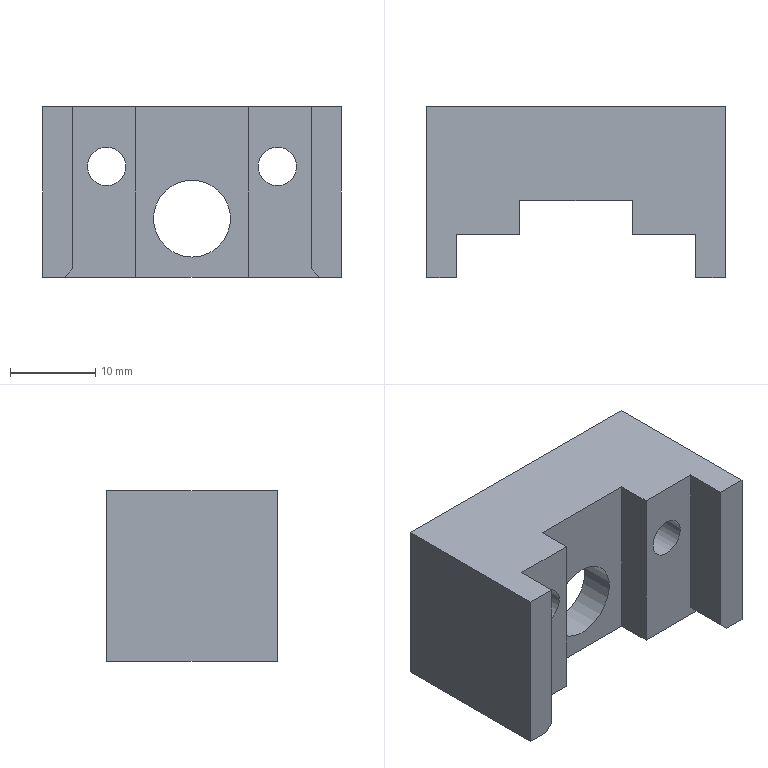Part | NX | features BREP 1 | 1 solid | 27 faces | box 35 x 20 x 20 mm | volume 7593 mm3 | plane 22 | cylinder 5 | commonest cylinder face diameters 4.5 x2 8 x2 9 x1
STEP:
#1=CARTESIAN_POINT('',(10.,-5.,-0.75));
#2=VERTEX_POINT('',#1);
#3=CARTESIAN_POINT('',(10.,-5.,-3.));
#4=DIRECTION('',(0.,1.,0.));
#5=DIRECTION('',(0.,0.,1.));
#6=AXIS2_PLACEMENT_3D('',#3,#4,#5);
#7=CIRCLE('',#6,2.25);
#8=EDGE_CURVE('',#2,#2,#7,.T.);
#9=ORIENTED_EDGE('',*,*,#8,.T.);
#10=EDGE_LOOP('',(#9));
#11=FACE_BOUND('',#10,.T.);
#12=CARTESIAN_POINT('',(14.,-5.,4.));
#13=VERTEX_POINT('',#12);
#14=CARTESIAN_POINT('',(6.6,-5.,4.));
#15=VERTEX_POINT('',#14);
#16=CARTESIAN_POINT('',(14.,-5.,4.));
#17=DIRECTION('',(-1.,0.,0.));
#18=VECTOR('',#17,1000.);
#19=LINE('',#16,#18);
#20=EDGE_CURVE('',#13,#15,#19,.T.);
#21=ORIENTED_EDGE('',*,*,#20,.T.);
#22=CARTESIAN_POINT('',(6.6,-5.,-16.));
#23=VERTEX_POINT('',#22);
#24=CARTESIAN_POINT('',(6.6,-5.,-16.));
#25=DIRECTION('',(0.,0.,1.));
#26=VECTOR('',#25,1000.);
#27=LINE('',#24,#26);
#28=EDGE_CURVE('',#23,#15,#27,.T.);
#29=ORIENTED_EDGE('',*,*,#28,.F.);
#30=CARTESIAN_POINT('',(15.,-5.,-16.));
#31=VERTEX_POINT('',#30);
#32=CARTESIAN_POINT('',(17.5,-5.,-16.));
#33=DIRECTION('',(1.,0.,0.));
#34=VECTOR('',#33,1000.);
#35=LINE('',#32,#34);
#36=EDGE_CURVE('',#23,#31,#35,.T.);
#37=ORIENTED_EDGE('',*,*,#36,.T.);
#38=CARTESIAN_POINT('',(14.,-5.,-15.));
#39=VERTEX_POINT('',#38);
#40=CARTESIAN_POINT('',(3.,-5.,-4.));
#41=DIRECTION('',(0.7071,0.,-0.7071));
#42=VECTOR('',#41,1000.);
#43=LINE('',#40,#42);
#44=EDGE_CURVE('',#39,#31,#43,.T.);
#45=ORIENTED_EDGE('',*,*,#44,.F.);
#46=CARTESIAN_POINT('',(14.,-5.,4.));
#47=DIRECTION('',(0.,0.,1.));
#48=VECTOR('',#47,1000.);
#49=LINE('',#46,#48);
#50=EDGE_CURVE('',#39,#13,#49,.T.);
#51=ORIENTED_EDGE('',*,*,#50,.T.);
#52=EDGE_LOOP('',(#21,#29,#37,#45,#51));
#53=FACE_BOUND('',#52,.T.);
#54=CARTESIAN_POINT('',(0.,-5.,0.));
#55=DIRECTION('',(0.,1.,0.));
#56=DIRECTION('',(0.,0.,-1.));
#57=AXIS2_PLACEMENT_3D('',#54,#55,#56);
#58=PLANE('',#57);
#59=ADVANCED_FACE('',(#11,#53),#58,.F.);
#60=CARTESIAN_POINT('',(0.,3.,-4.619));
#61=VERTEX_POINT('',#60);
#62=CARTESIAN_POINT('',(0.,3.,-9.119));
#63=DIRECTION('',(0.,1.,0.));
#64=DIRECTION('',(0.,0.,1.));
#65=AXIS2_PLACEMENT_3D('',#62,#63,#64);
#66=CIRCLE('',#65,4.5);
#67=EDGE_CURVE('',#61,#61,#66,.T.);
#68=ORIENTED_EDGE('',*,*,#67,.T.);
#69=EDGE_LOOP('',(#68));
#70=FACE_BOUND('',#69,.T.);
#71=CARTESIAN_POINT('',(0.,-1.,-13.619));
#72=VERTEX_POINT('',#71);
#73=CARTESIAN_POINT('',(0.,-1.,-9.119));
#74=DIRECTION('',(0.,1.,0.));
#75=DIRECTION('',(0.,0.,-1.));
#76=AXIS2_PLACEMENT_3D('',#73,#74,#75);
#77=CIRCLE('',#76,4.5);
#78=EDGE_CURVE('',#72,#72,#77,.T.);
#79=ORIENTED_EDGE('',*,*,#78,.F.);
#80=EDGE_LOOP('',(#79));
#81=FACE_BOUND('',#80,.T.);
#82=CARTESIAN_POINT('',(0.,3.,-9.119));
#83=DIRECTION('',(0.,1.,0.));
#84=DIRECTION('',(0.,0.,-1.));
#85=AXIS2_PLACEMENT_3D('',#82,#83,#84);
#86=CYLINDRICAL_SURFACE('',#85,4.5);
#87=ADVANCED_FACE('',(#70,#81),#86,.F.);
#88=CARTESIAN_POINT('',(3.,3.,-4.));
#89=VERTEX_POINT('',#88);
#90=CARTESIAN_POINT('',(15.,3.,-16.));
#91=VERTEX_POINT('',#90);
#92=CARTESIAN_POINT('',(3.,3.,-4.));
#93=DIRECTION('',(0.7071,0.,-0.7071));
#94=VECTOR('',#93,1000.);
#95=LINE('',#92,#94);
#96=EDGE_CURVE('',#89,#91,#95,.T.);
#97=ORIENTED_EDGE('',*,*,#96,.F.);
#98=CARTESIAN_POINT('',(3.,10.,-4.));
#99=VERTEX_POINT('',#98);
#100=CARTESIAN_POINT('',(3.,10.,-4.));
#101=DIRECTION('',(0.,-1.,0.));
#102=VECTOR('',#101,1000.);
#103=LINE('',#100,#102);
#104=EDGE_CURVE('',#99,#89,#103,.T.);
#105=ORIENTED_EDGE('',*,*,#104,.F.);
#106=CARTESIAN_POINT('',(15.,10.,-16.));
#107=VERTEX_POINT('',#106);
#108=CARTESIAN_POINT('',(3.,10.,-4.));
#109=DIRECTION('',(-0.7071,0.,0.7071));
#110=VECTOR('',#109,1000.);
#111=LINE('',#108,#110);
#112=EDGE_CURVE('',#107,#99,#111,.T.);
#113=ORIENTED_EDGE('',*,*,#112,.F.);
#114=CARTESIAN_POINT('',(15.,10.,-16.));
#115=DIRECTION('',(0.,-1.,0.));
#116=VECTOR('',#115,1000.);
#117=LINE('',#114,#116);
#118=EDGE_CURVE('',#107,#91,#117,.T.);
#119=ORIENTED_EDGE('',*,*,#118,.T.);
#120=EDGE_LOOP('',(#97,#105,#113,#119));
#121=FACE_BOUND('',#120,.T.);
#122=CARTESIAN_POINT('',(3.,10.,-4.));
#123=DIRECTION('',(0.7071,0.,0.7071));
#124=DIRECTION('',(-0.7071,0.,0.7071));
#125=AXIS2_PLACEMENT_3D('',#122,#123,#124);
#126=PLANE('',#125);
#127=ADVANCED_FACE('',(#121),#126,.F.);
#128=CARTESIAN_POINT('',(-3.,3.,-4.));
#129=VERTEX_POINT('',#128);
#130=CARTESIAN_POINT('',(17.5,3.,-4.));
#131=DIRECTION('',(-1.,0.,0.));
#132=VECTOR('',#131,1000.);
#133=LINE('',#130,#132);
#134=EDGE_CURVE('',#89,#129,#133,.T.);
#135=ORIENTED_EDGE('',*,*,#134,.T.);
#136=CARTESIAN_POINT('',(-3.,10.,-4.));
#137=VERTEX_POINT('',#136);
#138=CARTESIAN_POINT('',(-3.,10.,-4.));
#139=DIRECTION('',(0.,-1.,0.));
#140=VECTOR('',#139,1000.);
#141=LINE('',#138,#140);
#142=EDGE_CURVE('',#137,#129,#141,.T.);
#143=ORIENTED_EDGE('',*,*,#142,.F.);
#144=CARTESIAN_POINT('',(-3.,10.,-4.));
#145=DIRECTION('',(-1.,0.,0.));
#146=VECTOR('',#145,1000.);
#147=LINE('',#144,#146);
#148=EDGE_CURVE('',#99,#137,#147,.T.);
#149=ORIENTED_EDGE('',*,*,#148,.F.);
#150=ORIENTED_EDGE('',*,*,#104,.T.);
#151=EDGE_LOOP('',(#135,#143,#149,#150));
#152=FACE_BOUND('',#151,.T.);
#153=CARTESIAN_POINT('',(-3.,10.,-4.));
#154=DIRECTION('',(0.,0.,1.));
#155=DIRECTION('',(-1.,0.,0.));
#156=AXIS2_PLACEMENT_3D('',#153,#154,#155);
#157=PLANE('',#156);
#158=ADVANCED_FACE('',(#152),#157,.F.);
#159=CARTESIAN_POINT('',(-15.,3.,-16.));
#160=VERTEX_POINT('',#159);
#161=CARTESIAN_POINT('',(-15.,3.,-16.));
#162=DIRECTION('',(0.7071,0.,0.7071));
#163=VECTOR('',#162,1000.);
#164=LINE('',#161,#163);
#165=EDGE_CURVE('',#160,#129,#164,.T.);
#166=ORIENTED_EDGE('',*,*,#165,.F.);
#167=CARTESIAN_POINT('',(-15.,10.,-16.));
#168=VERTEX_POINT('',#167);
#169=CARTESIAN_POINT('',(-15.,10.,-16.));
#170=DIRECTION('',(0.,-1.,0.));
#171=VECTOR('',#170,1000.);
#172=LINE('',#169,#171);
#173=EDGE_CURVE('',#168,#160,#172,.T.);
#174=ORIENTED_EDGE('',*,*,#173,.F.);
#175=CARTESIAN_POINT('',(-15.,10.,-16.));
#176=DIRECTION('',(-0.7071,0.,-0.7071));
#177=VECTOR('',#176,1000.);
#178=LINE('',#175,#177);
#179=EDGE_CURVE('',#137,#168,#178,.T.);
#180=ORIENTED_EDGE('',*,*,#179,.F.);
#181=ORIENTED_EDGE('',*,*,#142,.T.);
#182=EDGE_LOOP('',(#166,#174,#180,#181));
#183=FACE_BOUND('',#182,.T.);
#184=CARTESIAN_POINT('',(-15.,10.,-16.));
#185=DIRECTION('',(-0.7071,0.,0.7071));
#186=DIRECTION('',(-0.7071,0.,-0.7071));
#187=AXIS2_PLACEMENT_3D('',#184,#185,#186);
#188=PLANE('',#187);
#189=ADVANCED_FACE('',(#183),#188,.F.);
#190=CARTESIAN_POINT('',(14.,-10.,-15.));
#191=VERTEX_POINT('',#190);
#192=CARTESIAN_POINT('',(14.,-10.,4.));
#193=VERTEX_POINT('',#192);
#194=CARTESIAN_POINT('',(14.,-10.,4.));
#195=DIRECTION('',(0.,0.,1.));
#196=VECTOR('',#195,1000.);
#197=LINE('',#194,#196);
#198=EDGE_CURVE('',#191,#193,#197,.T.);
#199=ORIENTED_EDGE('',*,*,#198,.F.);
#200=CARTESIAN_POINT('',(15.,-10.,-16.));
#201=VERTEX_POINT('',#200);
#202=CARTESIAN_POINT('',(3.,-10.,-4.));
#203=DIRECTION('',(-0.7071,0.,0.7071));
#204=VECTOR('',#203,1000.);
#205=LINE('',#202,#204);
#206=EDGE_CURVE('',#201,#191,#205,.T.);
#207=ORIENTED_EDGE('',*,*,#206,.F.);
#208=CARTESIAN_POINT('',(17.5,-10.,-16.));
#209=VERTEX_POINT('',#208);
#210=CARTESIAN_POINT('',(15.,-10.,-16.));
#211=DIRECTION('',(-1.,0.,0.));
#212=VECTOR('',#211,1000.);
#213=LINE('',#210,#212);
#214=EDGE_CURVE('',#209,#201,#213,.T.);
#215=ORIENTED_EDGE('',*,*,#214,.F.);
#216=CARTESIAN_POINT('',(17.5,-10.,4.));
#217=VERTEX_POINT('',#216);
#218=CARTESIAN_POINT('',(17.5,-10.,-16.));
#219=DIRECTION('',(0.,0.,-1.));
#220=VECTOR('',#219,1000.);
#221=LINE('',#218,#220);
#222=EDGE_CURVE('',#217,#209,#221,.T.);
#223=ORIENTED_EDGE('',*,*,#222,.F.);
#224=CARTESIAN_POINT('',(17.5,-10.,4.));
#225=DIRECTION('',(1.,0.,0.));
#226=VECTOR('',#225,1000.);
#227=LINE('',#224,#226);
#228=EDGE_CURVE('',#193,#217,#227,.T.);
#229=ORIENTED_EDGE('',*,*,#228,.F.);
#230=EDGE_LOOP('',(#199,#207,#215,#223,#229));
#231=FACE_BOUND('',#230,.T.);
#232=CARTESIAN_POINT('',(0.,-10.,0.));
#233=DIRECTION('',(0.,-1.,0.));
#234=DIRECTION('',(0.,0.,1.));
#235=AXIS2_PLACEMENT_3D('',#232,#233,#234);
#236=PLANE('',#235);
#237=ADVANCED_FACE('',(#231),#236,.T.);
#238=CARTESIAN_POINT('',(-17.5,10.,-16.));
#239=VERTEX_POINT('',#238);
#240=CARTESIAN_POINT('',(-17.5,-10.,-16.));
#241=VERTEX_POINT('',#240);
#242=CARTESIAN_POINT('',(-17.5,10.,-16.));
#243=DIRECTION('',(0.,-1.,0.));
#244=VECTOR('',#243,1000.);
#245=LINE('',#242,#244);
#246=EDGE_CURVE('',#239,#241,#245,.T.);
#247=ORIENTED_EDGE('',*,*,#246,.T.);
#248=CARTESIAN_POINT('',(-17.5,-10.,4.));
#249=VERTEX_POINT('',#248);
#250=CARTESIAN_POINT('',(-17.5,-10.,4.));
#251=DIRECTION('',(0.,0.,1.));
#252=VECTOR('',#251,1000.);
#253=LINE('',#250,#252);
#254=EDGE_CURVE('',#241,#249,#253,.T.);
#255=ORIENTED_EDGE('',*,*,#254,.T.);
#256=CARTESIAN_POINT('',(-17.5,10.,4.));
#257=VERTEX_POINT('',#256);
#258=CARTESIAN_POINT('',(-17.5,10.,4.));
#259=DIRECTION('',(0.,-1.,0.));
#260=VECTOR('',#259,1000.);
#261=LINE('',#258,#260);
#262=EDGE_CURVE('',#257,#249,#261,.T.);
#263=ORIENTED_EDGE('',*,*,#262,.F.);
#264=CARTESIAN_POINT('',(-17.5,10.,4.));
#265=DIRECTION('',(0.,0.,1.));
#266=VECTOR('',#265,1000.);
#267=LINE('',#264,#266);
#268=EDGE_CURVE('',#239,#257,#267,.T.);
#269=ORIENTED_EDGE('',*,*,#268,.F.);
#270=EDGE_LOOP('',(#247,#255,#263,#269));
#271=FACE_BOUND('',#270,.T.);
#272=CARTESIAN_POINT('',(-17.5,10.,4.));
#273=DIRECTION('',(1.,0.,0.));
#274=DIRECTION('',(0.,0.,1.));
#275=AXIS2_PLACEMENT_3D('',#272,#273,#274);
#276=PLANE('',#275);
#277=ADVANCED_FACE('',(#271),#276,.F.);
#278=CARTESIAN_POINT('',(6.6,-1.,4.));
#279=VERTEX_POINT('',#278);
#280=CARTESIAN_POINT('',(-6.6,-1.,4.));
#281=VERTEX_POINT('',#280);
#282=CARTESIAN_POINT('',(6.6,-1.,4.));
#283=DIRECTION('',(-1.,0.,0.));
#284=VECTOR('',#283,1000.);
#285=LINE('',#282,#284);
#286=EDGE_CURVE('',#279,#281,#285,.T.);
#287=ORIENTED_EDGE('',*,*,#286,.F.);
#288=CARTESIAN_POINT('',(6.6,-1.,4.));
#289=DIRECTION('',(0.,-1.,0.));
#290=VECTOR('',#289,1000.);
#291=LINE('',#288,#290);
#292=EDGE_CURVE('',#279,#15,#291,.T.);
#293=ORIENTED_EDGE('',*,*,#292,.T.);
#294=ORIENTED_EDGE('',*,*,#20,.F.);
#295=CARTESIAN_POINT('',(14.,-5.,4.));
#296=DIRECTION('',(0.,-1.,0.));
#297=VECTOR('',#296,1000.);
#298=LINE('',#295,#297);
#299=EDGE_CURVE('',#13,#193,#298,.T.);
#300=ORIENTED_EDGE('',*,*,#299,.T.);
#301=ORIENTED_EDGE('',*,*,#228,.T.);
#302=CARTESIAN_POINT('',(17.5,10.,4.));
#303=VERTEX_POINT('',#302);
#304=CARTESIAN_POINT('',(17.5,10.,4.));
#305=DIRECTION('',(0.,-1.,0.));
#306=VECTOR('',#305,1000.);
#307=LINE('',#304,#306);
#308=EDGE_CURVE('',#303,#217,#307,.T.);
#309=ORIENTED_EDGE('',*,*,#308,.F.);
#310=CARTESIAN_POINT('',(17.5,10.,4.));
#311=DIRECTION('',(1.,0.,0.));
#312=VECTOR('',#311,1000.);
#313=LINE('',#310,#312);
#314=EDGE_CURVE('',#257,#303,#313,.T.);
#315=ORIENTED_EDGE('',*,*,#314,.F.);
#316=ORIENTED_EDGE('',*,*,#262,.T.);
#317=CARTESIAN_POINT('',(-14.,-10.,4.));
#318=VERTEX_POINT('',#317);
#319=CARTESIAN_POINT('',(17.5,-10.,4.));
#320=DIRECTION('',(1.,0.,0.));
#321=VECTOR('',#320,1000.);
#322=LINE('',#319,#321);
#323=EDGE_CURVE('',#249,#318,#322,.T.);
#324=ORIENTED_EDGE('',*,*,#323,.T.);
#325=CARTESIAN_POINT('',(-14.,-5.,4.));
#326=VERTEX_POINT('',#325);
#327=CARTESIAN_POINT('',(-14.,-5.,4.));
#328=DIRECTION('',(0.,-1.,0.));
#329=VECTOR('',#328,1000.);
#330=LINE('',#327,#329);
#331=EDGE_CURVE('',#326,#318,#330,.T.);
#332=ORIENTED_EDGE('',*,*,#331,.F.);
#333=CARTESIAN_POINT('',(-6.6,-5.,4.));
#334=VERTEX_POINT('',#333);
#335=CARTESIAN_POINT('',(14.,-5.,4.));
#336=DIRECTION('',(-1.,0.,0.));
#337=VECTOR('',#336,1000.);
#338=LINE('',#335,#337);
#339=EDGE_CURVE('',#334,#326,#338,.T.);
#340=ORIENTED_EDGE('',*,*,#339,.F.);
#341=CARTESIAN_POINT('',(-6.6,-1.,4.));
#342=DIRECTION('',(0.,-1.,0.));
#343=VECTOR('',#342,1000.);
#344=LINE('',#341,#343);
#345=EDGE_CURVE('',#281,#334,#344,.T.);
#346=ORIENTED_EDGE('',*,*,#345,.F.);
#347=EDGE_LOOP('',(#287,#293,#294,#300,#301,#309,#315,#316,#324,#332,#340,#346));
#348=FACE_BOUND('',#347,.T.);
#349=CARTESIAN_POINT('',(17.5,10.,4.));
#350=DIRECTION('',(0.,0.,-1.));
#351=DIRECTION('',(1.,0.,0.));
#352=AXIS2_PLACEMENT_3D('',#349,#350,#351);
#353=PLANE('',#352);
#354=ADVANCED_FACE('',(#348),#353,.F.);
#355=ORIENTED_EDGE('',*,*,#222,.T.);
#356=CARTESIAN_POINT('',(17.5,10.,-16.));
#357=VERTEX_POINT('',#356);
#358=CARTESIAN_POINT('',(17.5,10.,-16.));
#359=DIRECTION('',(0.,-1.,0.));
#360=VECTOR('',#359,1000.);
#361=LINE('',#358,#360);
#362=EDGE_CURVE('',#357,#209,#361,.T.);
#363=ORIENTED_EDGE('',*,*,#362,.F.);
#364=CARTESIAN_POINT('',(17.5,10.,-16.));
#365=DIRECTION('',(0.,0.,-1.));
#366=VECTOR('',#365,1000.);
#367=LINE('',#364,#366);
#368=EDGE_CURVE('',#303,#357,#367,.T.);
#369=ORIENTED_EDGE('',*,*,#368,.F.);
#370=ORIENTED_EDGE('',*,*,#308,.T.);
#371=EDGE_LOOP('',(#355,#363,#369,#370));
#372=FACE_BOUND('',#371,.T.);
#373=CARTESIAN_POINT('',(17.5,10.,-16.));
#374=DIRECTION('',(-1.,0.,0.));
#375=DIRECTION('',(0.,0.,-1.));
#376=AXIS2_PLACEMENT_3D('',#373,#374,#375);
#377=PLANE('',#376);
#378=ADVANCED_FACE('',(#372),#377,.F.);
#379=ORIENTED_EDGE('',*,*,#36,.F.);
#380=CARTESIAN_POINT('',(6.6,-1.,-16.));
#381=VERTEX_POINT('',#380);
#382=CARTESIAN_POINT('',(6.6,-1.,-16.));
#383=DIRECTION('',(0.,-1.,0.));
#384=VECTOR('',#383,1000.);
#385=LINE('',#382,#384);
#386=EDGE_CURVE('',#381,#23,#385,.T.);
#387=ORIENTED_EDGE('',*,*,#386,.F.);
#388=CARTESIAN_POINT('',(-6.6,-1.,-16.));
#389=VERTEX_POINT('',#388);
#390=CARTESIAN_POINT('',(6.6,-1.,-16.));
#391=DIRECTION('',(1.,0.,0.));
#392=VECTOR('',#391,1000.);
#393=LINE('',#390,#392);
#394=EDGE_CURVE('',#389,#381,#393,.T.);
#395=ORIENTED_EDGE('',*,*,#394,.F.);
#396=CARTESIAN_POINT('',(-6.6,-5.,-16.));
#397=VERTEX_POINT('',#396);
#398=CARTESIAN_POINT('',(-6.6,-1.,-16.));
#399=DIRECTION('',(0.,-1.,0.));
#400=VECTOR('',#399,1000.);
#401=LINE('',#398,#400);
#402=EDGE_CURVE('',#389,#397,#401,.T.);
#403=ORIENTED_EDGE('',*,*,#402,.T.);
#404=CARTESIAN_POINT('',(-15.,-5.,-16.));
#405=VERTEX_POINT('',#404);
#406=CARTESIAN_POINT('',(17.5,-5.,-16.));
#407=DIRECTION('',(1.,0.,0.));
#408=VECTOR('',#407,1000.);
#409=LINE('',#406,#408);
#410=EDGE_CURVE('',#405,#397,#409,.T.);
#411=ORIENTED_EDGE('',*,*,#410,.F.);
#412=CARTESIAN_POINT('',(-15.,-10.,-16.));
#413=VERTEX_POINT('',#412);
#414=CARTESIAN_POINT('',(-15.,10.,-16.));
#415=DIRECTION('',(0.,-1.,0.));
#416=VECTOR('',#415,1000.);
#417=LINE('',#414,#416);
#418=EDGE_CURVE('',#405,#413,#417,.T.);
#419=ORIENTED_EDGE('',*,*,#418,.T.);
#420=CARTESIAN_POINT('',(-17.5,-10.,-16.));
#421=DIRECTION('',(-1.,0.,0.));
#422=VECTOR('',#421,1000.);
#423=LINE('',#420,#422);
#424=EDGE_CURVE('',#413,#241,#423,.T.);
#425=ORIENTED_EDGE('',*,*,#424,.T.);
#426=ORIENTED_EDGE('',*,*,#246,.F.);
#427=CARTESIAN_POINT('',(-17.5,10.,-16.));
#428=DIRECTION('',(-1.,0.,0.));
#429=VECTOR('',#428,1000.);
#430=LINE('',#427,#429);
#431=EDGE_CURVE('',#168,#239,#430,.T.);
#432=ORIENTED_EDGE('',*,*,#431,.F.);
#433=ORIENTED_EDGE('',*,*,#173,.T.);
#434=CARTESIAN_POINT('',(17.5,3.,-16.));
#435=DIRECTION('',(1.,0.,0.));
#436=VECTOR('',#435,1000.);
#437=LINE('',#434,#436);
#438=EDGE_CURVE('',#160,#91,#437,.T.);
#439=ORIENTED_EDGE('',*,*,#438,.T.);
#440=ORIENTED_EDGE('',*,*,#118,.F.);
#441=CARTESIAN_POINT('',(15.,10.,-16.));
#442=DIRECTION('',(-1.,0.,0.));
#443=VECTOR('',#442,1000.);
#444=LINE('',#441,#443);
#445=EDGE_CURVE('',#357,#107,#444,.T.);
#446=ORIENTED_EDGE('',*,*,#445,.F.);
#447=ORIENTED_EDGE('',*,*,#362,.T.);
#448=ORIENTED_EDGE('',*,*,#214,.T.);
#449=CARTESIAN_POINT('',(15.,10.,-16.));
#450=DIRECTION('',(0.,-1.,0.));
#451=VECTOR('',#450,1000.);
#452=LINE('',#449,#451);
#453=EDGE_CURVE('',#31,#201,#452,.T.);
#454=ORIENTED_EDGE('',*,*,#453,.F.);
#455=EDGE_LOOP('',(#379,#387,#395,#403,#411,#419,#425,#426,#432,#433,#439,#440,#446,#447,#448,#454));
#456=FACE_BOUND('',#455,.T.);
#457=CARTESIAN_POINT('',(15.,10.,-16.));
#458=DIRECTION('',(0.,0.,1.));
#459=DIRECTION('',(-1.,0.,0.));
#460=AXIS2_PLACEMENT_3D('',#457,#458,#459);
#461=PLANE('',#460);
#462=ADVANCED_FACE('',(#456),#461,.F.);
#463=CARTESIAN_POINT('',(14.,-5.,-15.));
#464=DIRECTION('',(0.,-1.,0.));
#465=VECTOR('',#464,1000.);
#466=LINE('',#463,#465);
#467=EDGE_CURVE('',#39,#191,#466,.T.);
#468=ORIENTED_EDGE('',*,*,#467,.F.);
#469=ORIENTED_EDGE('',*,*,#44,.T.);
#470=ORIENTED_EDGE('',*,*,#453,.T.);
#471=ORIENTED_EDGE('',*,*,#206,.T.);
#472=EDGE_LOOP('',(#468,#469,#470,#471));
#473=FACE_BOUND('',#472,.T.);
#474=CARTESIAN_POINT('',(3.,10.,-4.));
#475=DIRECTION('',(0.7071,0.,0.7071));
#476=DIRECTION('',(-0.7071,0.,0.7071));
#477=AXIS2_PLACEMENT_3D('',#474,#475,#476);
#478=PLANE('',#477);
#479=ADVANCED_FACE('',(#473),#478,.F.);
#480=ORIENTED_EDGE('',*,*,#418,.F.);
#481=CARTESIAN_POINT('',(-14.,-5.,-15.));
#482=VERTEX_POINT('',#481);
#483=CARTESIAN_POINT('',(-15.,-5.,-16.));
#484=DIRECTION('',(0.7071,0.,0.7071));
#485=VECTOR('',#484,1000.);
#486=LINE('',#483,#485);
#487=EDGE_CURVE('',#405,#482,#486,.T.);
#488=ORIENTED_EDGE('',*,*,#487,.T.);
#489=CARTESIAN_POINT('',(-14.,-10.,-15.));
#490=VERTEX_POINT('',#489);
#491=CARTESIAN_POINT('',(-14.,-5.,-15.));
#492=DIRECTION('',(0.,-1.,0.));
#493=VECTOR('',#492,1000.);
#494=LINE('',#491,#493);
#495=EDGE_CURVE('',#482,#490,#494,.T.);
#496=ORIENTED_EDGE('',*,*,#495,.T.);
#497=CARTESIAN_POINT('',(-15.,-10.,-16.));
#498=DIRECTION('',(-0.7071,0.,-0.7071));
#499=VECTOR('',#498,1000.);
#500=LINE('',#497,#499);
#501=EDGE_CURVE('',#490,#413,#500,.T.);
#502=ORIENTED_EDGE('',*,*,#501,.T.);
#503=EDGE_LOOP('',(#480,#488,#496,#502));
#504=FACE_BOUND('',#503,.T.);
#505=CARTESIAN_POINT('',(-15.,10.,-16.));
#506=DIRECTION('',(-0.7071,0.,0.7071));
#507=DIRECTION('',(-0.7071,0.,-0.7071));
#508=AXIS2_PLACEMENT_3D('',#505,#506,#507);
#509=PLANE('',#508);
#510=ADVANCED_FACE('',(#504),#509,.F.);
#511=CARTESIAN_POINT('',(-10.,10.,1.));
#512=VERTEX_POINT('',#511);
#513=CARTESIAN_POINT('',(-10.,10.,-3.));
#514=DIRECTION('',(0.,1.,0.));
#515=DIRECTION('',(0.,0.,1.));
#516=AXIS2_PLACEMENT_3D('',#513,#514,#515);
#517=CIRCLE('',#516,4.);
#518=EDGE_CURVE('',#512,#512,#517,.T.);
#519=ORIENTED_EDGE('',*,*,#518,.F.);
#520=EDGE_LOOP('',(#519));
#521=FACE_BOUND('',#520,.T.);
#522=CARTESIAN_POINT('',(10.,10.,1.));
#523=VERTEX_POINT('',#522);
#524=CARTESIAN_POINT('',(10.,10.,-3.));
#525=DIRECTION('',(0.,1.,0.));
#526=DIRECTION('',(0.,0.,1.));
#527=AXIS2_PLACEMENT_3D('',#524,#525,#526);
#528=CIRCLE('',#527,4.);
#529=EDGE_CURVE('',#523,#523,#528,.T.);
#530=ORIENTED_EDGE('',*,*,#529,.F.);
#531=EDGE_LOOP('',(#530));
#532=FACE_BOUND('',#531,.T.);
#533=ORIENTED_EDGE('',*,*,#431,.T.);
#534=ORIENTED_EDGE('',*,*,#268,.T.);
#535=ORIENTED_EDGE('',*,*,#314,.T.);
#536=ORIENTED_EDGE('',*,*,#368,.T.);
#537=ORIENTED_EDGE('',*,*,#445,.T.);
#538=ORIENTED_EDGE('',*,*,#112,.T.);
#539=ORIENTED_EDGE('',*,*,#148,.T.);
#540=ORIENTED_EDGE('',*,*,#179,.T.);
#541=EDGE_LOOP('',(#533,#534,#535,#536,#537,#538,#539,#540));
#542=FACE_BOUND('',#541,.T.);
#543=CARTESIAN_POINT('',(0.,10.,0.));
#544=DIRECTION('',(0.,-1.,0.));
#545=DIRECTION('',(0.,0.,1.));
#546=AXIS2_PLACEMENT_3D('',#543,#544,#545);
#547=PLANE('',#546);
#548=ADVANCED_FACE('',(#521,#532,#542),#547,.F.);
#549=CARTESIAN_POINT('',(-14.,-10.,4.));
#550=DIRECTION('',(0.,0.,-1.));
#551=VECTOR('',#550,1000.);
#552=LINE('',#549,#551);
#553=EDGE_CURVE('',#318,#490,#552,.T.);
#554=ORIENTED_EDGE('',*,*,#553,.F.);
#555=ORIENTED_EDGE('',*,*,#323,.F.);
#556=ORIENTED_EDGE('',*,*,#254,.F.);
#557=ORIENTED_EDGE('',*,*,#424,.F.);
#558=ORIENTED_EDGE('',*,*,#501,.F.);
#559=EDGE_LOOP('',(#554,#555,#556,#557,#558));
#560=FACE_BOUND('',#559,.T.);
#561=CARTESIAN_POINT('',(0.,-10.,0.));
#562=DIRECTION('',(0.,-1.,0.));
#563=DIRECTION('',(0.,0.,1.));
#564=AXIS2_PLACEMENT_3D('',#561,#562,#563);
#565=PLANE('',#564);
#566=ADVANCED_FACE('',(#560),#565,.T.);
#567=CARTESIAN_POINT('',(-10.,-5.,-0.75));
#568=VERTEX_POINT('',#567);
#569=CARTESIAN_POINT('',(-10.,-5.,-3.));
#570=DIRECTION('',(0.,1.,0.));
#571=DIRECTION('',(0.,0.,1.));
#572=AXIS2_PLACEMENT_3D('',#569,#570,#571);
#573=CIRCLE('',#572,2.25);
#574=EDGE_CURVE('',#568,#568,#573,.T.);
#575=ORIENTED_EDGE('',*,*,#574,.T.);
#576=EDGE_LOOP('',(#575));
#577=FACE_BOUND('',#576,.T.);
#578=ORIENTED_EDGE('',*,*,#410,.T.);
#579=CARTESIAN_POINT('',(-6.6,-5.,-16.));
#580=DIRECTION('',(0.,0.,-1.));
#581=VECTOR('',#580,1000.);
#582=LINE('',#579,#581);
#583=EDGE_CURVE('',#334,#397,#582,.T.);
#584=ORIENTED_EDGE('',*,*,#583,.F.);
#585=ORIENTED_EDGE('',*,*,#339,.T.);
#586=CARTESIAN_POINT('',(-14.,-5.,4.));
#587=DIRECTION('',(0.,0.,-1.));
#588=VECTOR('',#587,1000.);
#589=LINE('',#586,#588);
#590=EDGE_CURVE('',#326,#482,#589,.T.);
#591=ORIENTED_EDGE('',*,*,#590,.T.);
#592=ORIENTED_EDGE('',*,*,#487,.F.);
#593=EDGE_LOOP('',(#578,#584,#585,#591,#592));
#594=FACE_BOUND('',#593,.T.);
#595=CARTESIAN_POINT('',(0.,-5.,0.));
#596=DIRECTION('',(0.,1.,0.));
#597=DIRECTION('',(0.,0.,-1.));
#598=AXIS2_PLACEMENT_3D('',#595,#596,#597);
#599=PLANE('',#598);
#600=ADVANCED_FACE('',(#577,#594),#599,.F.);
#601=ORIENTED_EDGE('',*,*,#198,.T.);
#602=ORIENTED_EDGE('',*,*,#299,.F.);
#603=ORIENTED_EDGE('',*,*,#50,.F.);
#604=ORIENTED_EDGE('',*,*,#467,.T.);
#605=EDGE_LOOP('',(#601,#602,#603,#604));
#606=FACE_BOUND('',#605,.T.);
#607=CARTESIAN_POINT('',(14.,-5.,4.));
#608=DIRECTION('',(1.,0.,0.));
#609=DIRECTION('',(0.,0.,1.));
#610=AXIS2_PLACEMENT_3D('',#607,#608,#609);
#611=PLANE('',#610);
#612=ADVANCED_FACE('',(#606),#611,.F.);
#613=ORIENTED_EDGE('',*,*,#553,.T.);
#614=ORIENTED_EDGE('',*,*,#495,.F.);
#615=ORIENTED_EDGE('',*,*,#590,.F.);
#616=ORIENTED_EDGE('',*,*,#331,.T.);
#617=EDGE_LOOP('',(#613,#614,#615,#616));
#618=FACE_BOUND('',#617,.T.);
#619=CARTESIAN_POINT('',(-14.,-5.,4.));
#620=DIRECTION('',(-1.,0.,0.));
#621=DIRECTION('',(0.,0.,-1.));
#622=AXIS2_PLACEMENT_3D('',#619,#620,#621);
#623=PLANE('',#622);
#624=ADVANCED_FACE('',(#618),#623,.F.);
#625=ORIENTED_EDGE('',*,*,#67,.F.);
#626=EDGE_LOOP('',(#625));
#627=FACE_BOUND('',#626,.T.);
#628=ORIENTED_EDGE('',*,*,#134,.F.);
#629=ORIENTED_EDGE('',*,*,#96,.T.);
#630=ORIENTED_EDGE('',*,*,#438,.F.);
#631=ORIENTED_EDGE('',*,*,#165,.T.);
#632=EDGE_LOOP('',(#628,#629,#630,#631));
#633=FACE_BOUND('',#632,.T.);
#634=CARTESIAN_POINT('',(0.,3.,0.));
#635=DIRECTION('',(0.,-1.,0.));
#636=DIRECTION('',(0.,0.,1.));
#637=AXIS2_PLACEMENT_3D('',#634,#635,#636);
#638=PLANE('',#637);
#639=ADVANCED_FACE('',(#627,#633),#638,.F.);
#640=CARTESIAN_POINT('',(6.6,-1.,-16.));
#641=DIRECTION('',(0.,0.,1.));
#642=VECTOR('',#641,1000.);
#643=LINE('',#640,#642);
#644=EDGE_CURVE('',#381,#279,#643,.T.);
#645=ORIENTED_EDGE('',*,*,#644,.T.);
#646=ORIENTED_EDGE('',*,*,#286,.T.);
#647=CARTESIAN_POINT('',(-6.6,-1.,-16.));
#648=DIRECTION('',(0.,0.,-1.));
#649=VECTOR('',#648,1000.);
#650=LINE('',#647,#649);
#651=EDGE_CURVE('',#281,#389,#650,.T.);
#652=ORIENTED_EDGE('',*,*,#651,.T.);
#653=ORIENTED_EDGE('',*,*,#394,.T.);
#654=EDGE_LOOP('',(#645,#646,#652,#653));
#655=FACE_BOUND('',#654,.T.);
#656=ORIENTED_EDGE('',*,*,#78,.T.);
#657=EDGE_LOOP('',(#656));
#658=FACE_BOUND('',#657,.T.);
#659=CARTESIAN_POINT('',(0.,-1.,0.));
#660=DIRECTION('',(0.,-1.,0.));
#661=DIRECTION('',(0.,0.,1.));
#662=AXIS2_PLACEMENT_3D('',#659,#660,#661);
#663=PLANE('',#662);
#664=ADVANCED_FACE('',(#655,#658),#663,.T.);
#665=ORIENTED_EDGE('',*,*,#28,.T.);
#666=ORIENTED_EDGE('',*,*,#292,.F.);
#667=ORIENTED_EDGE('',*,*,#644,.F.);
#668=ORIENTED_EDGE('',*,*,#386,.T.);
#669=EDGE_LOOP('',(#665,#666,#667,#668));
#670=FACE_BOUND('',#669,.T.);
#671=CARTESIAN_POINT('',(6.6,-1.,-16.));
#672=DIRECTION('',(1.,0.,0.));
#673=DIRECTION('',(0.,0.,1.));
#674=AXIS2_PLACEMENT_3D('',#671,#672,#673);
#675=PLANE('',#674);
#676=ADVANCED_FACE('',(#670),#675,.F.);
#677=ORIENTED_EDGE('',*,*,#583,.T.);
#678=ORIENTED_EDGE('',*,*,#402,.F.);
#679=ORIENTED_EDGE('',*,*,#651,.F.);
#680=ORIENTED_EDGE('',*,*,#345,.T.);
#681=EDGE_LOOP('',(#677,#678,#679,#680));
#682=FACE_BOUND('',#681,.T.);
#683=CARTESIAN_POINT('',(-6.6,-1.,-16.));
#684=DIRECTION('',(-1.,0.,0.));
#685=DIRECTION('',(0.,0.,-1.));
#686=AXIS2_PLACEMENT_3D('',#683,#684,#685);
#687=PLANE('',#686);
#688=ADVANCED_FACE('',(#682),#687,.F.);
#689=CARTESIAN_POINT('',(10.,5.6,-0.75));
#690=VERTEX_POINT('',#689);
#691=CARTESIAN_POINT('',(10.,5.6,-3.));
#692=DIRECTION('',(0.,1.,0.));
#693=DIRECTION('',(0.,0.,1.));
#694=AXIS2_PLACEMENT_3D('',#691,#692,#693);
#695=CIRCLE('',#694,2.25);
#696=EDGE_CURVE('',#690,#690,#695,.T.);
#697=ORIENTED_EDGE('',*,*,#696,.T.);
#698=EDGE_LOOP('',(#697));
#699=FACE_BOUND('',#698,.T.);
#700=ORIENTED_EDGE('',*,*,#8,.F.);
#701=EDGE_LOOP('',(#700));
#702=FACE_BOUND('',#701,.T.);
#703=CARTESIAN_POINT('',(10.,10.,-3.));
#704=DIRECTION('',(0.,1.,0.));
#705=DIRECTION('',(0.,0.,-1.));
#706=AXIS2_PLACEMENT_3D('',#703,#704,#705);
#707=CYLINDRICAL_SURFACE('',#706,2.25);
#708=ADVANCED_FACE('',(#699,#702),#707,.F.);
#709=ORIENTED_EDGE('',*,*,#696,.F.);
#710=EDGE_LOOP('',(#709));
#711=FACE_BOUND('',#710,.T.);
#712=CARTESIAN_POINT('',(10.,5.6,1.));
#713=VERTEX_POINT('',#712);
#714=CARTESIAN_POINT('',(10.,5.6,-3.));
#715=DIRECTION('',(0.,1.,0.));
#716=DIRECTION('',(0.,0.,1.));
#717=AXIS2_PLACEMENT_3D('',#714,#715,#716);
#718=CIRCLE('',#717,4.);
#719=EDGE_CURVE('',#713,#713,#718,.T.);
#720=ORIENTED_EDGE('',*,*,#719,.T.);
#721=EDGE_LOOP('',(#720));
#722=FACE_BOUND('',#721,.T.);
#723=CARTESIAN_POINT('',(12.25,5.6,-3.));
#724=DIRECTION('',(0.,-1.,0.));
#725=DIRECTION('',(0.,0.,1.));
#726=AXIS2_PLACEMENT_3D('',#723,#724,#725);
#727=PLANE('',#726);
#728=ADVANCED_FACE('',(#711,#722),#727,.F.);
#729=ORIENTED_EDGE('',*,*,#719,.F.);
#730=EDGE_LOOP('',(#729));
#731=FACE_BOUND('',#730,.T.);
#732=ORIENTED_EDGE('',*,*,#529,.T.);
#733=EDGE_LOOP('',(#732));
#734=FACE_BOUND('',#733,.T.);
#735=CARTESIAN_POINT('',(10.,10.,-3.));
#736=DIRECTION('',(0.,1.,0.));
#737=DIRECTION('',(0.,0.,-1.));
#738=AXIS2_PLACEMENT_3D('',#735,#736,#737);
#739=CYLINDRICAL_SURFACE('',#738,4.);
#740=ADVANCED_FACE('',(#731,#734),#739,.F.);
#741=CARTESIAN_POINT('',(-10.,5.6,-0.75));
#742=VERTEX_POINT('',#741);
#743=CARTESIAN_POINT('',(-10.,5.6,-3.));
#744=DIRECTION('',(0.,1.,0.));
#745=DIRECTION('',(0.,0.,1.));
#746=AXIS2_PLACEMENT_3D('',#743,#744,#745);
#747=CIRCLE('',#746,2.25);
#748=EDGE_CURVE('',#742,#742,#747,.T.);
#749=ORIENTED_EDGE('',*,*,#748,.T.);
#750=EDGE_LOOP('',(#749));
#751=FACE_BOUND('',#750,.T.);
#752=ORIENTED_EDGE('',*,*,#574,.F.);
#753=EDGE_LOOP('',(#752));
#754=FACE_BOUND('',#753,.T.);
#755=CARTESIAN_POINT('',(-10.,10.,-3.));
#756=DIRECTION('',(0.,1.,0.));
#757=DIRECTION('',(0.,0.,-1.));
#758=AXIS2_PLACEMENT_3D('',#755,#756,#757);
#759=CYLINDRICAL_SURFACE('',#758,2.25);
#760=ADVANCED_FACE('',(#751,#754),#759,.F.);
#761=ORIENTED_EDGE('',*,*,#748,.F.);
#762=EDGE_LOOP('',(#761));
#763=FACE_BOUND('',#762,.T.);
#764=CARTESIAN_POINT('',(-10.,5.6,1.));
#765=VERTEX_POINT('',#764);
#766=CARTESIAN_POINT('',(-10.,5.6,-3.));
#767=DIRECTION('',(0.,1.,0.));
#768=DIRECTION('',(0.,0.,1.));
#769=AXIS2_PLACEMENT_3D('',#766,#767,#768);
#770=CIRCLE('',#769,4.);
#771=EDGE_CURVE('',#765,#765,#770,.T.);
#772=ORIENTED_EDGE('',*,*,#771,.T.);
#773=EDGE_LOOP('',(#772));
#774=FACE_BOUND('',#773,.T.);
#775=CARTESIAN_POINT('',(-7.75,5.6,-3.));
#776=DIRECTION('',(0.,-1.,0.));
#777=DIRECTION('',(0.,0.,1.));
#778=AXIS2_PLACEMENT_3D('',#775,#776,#777);
#779=PLANE('',#778);
#780=ADVANCED_FACE('',(#763,#774),#779,.F.);
#781=ORIENTED_EDGE('',*,*,#771,.F.);
#782=EDGE_LOOP('',(#781));
#783=FACE_BOUND('',#782,.T.);
#784=ORIENTED_EDGE('',*,*,#518,.T.);
#785=EDGE_LOOP('',(#784));
#786=FACE_BOUND('',#785,.T.);
#787=CARTESIAN_POINT('',(-10.,10.,-3.));
#788=DIRECTION('',(0.,1.,0.));
#789=DIRECTION('',(0.,0.,-1.));
#790=AXIS2_PLACEMENT_3D('',#787,#788,#789);
#791=CYLINDRICAL_SURFACE('',#790,4.);
#792=ADVANCED_FACE('',(#783,#786),#791,.F.);
#793=CLOSED_SHELL('',(#59,#87,#127,#158,#189,#237,#277,#354,#378,#462,#479,#510,#548,#566,#600,#612,#624,#639,#664,#676,#688,#708,#728,#740,#760,#780,#792));
#794=MANIFOLD_SOLID_BREP('',#793);
#795=(LENGTH_UNIT()NAMED_UNIT(*)SI_UNIT(.MILLI.,.METRE.));
#796=UNCERTAINTY_MEASURE_WITH_UNIT(LENGTH_MEASURE(0.00001),#795,'','');
#797=(NAMED_UNIT(*)PLANE_ANGLE_UNIT()SI_UNIT($,.RADIAN.));
#798=(NAMED_UNIT(*)SI_UNIT($,.STERADIAN.)SOLID_ANGLE_UNIT());
#799=(GEOMETRIC_REPRESENTATION_CONTEXT(3)GLOBAL_UNCERTAINTY_ASSIGNED_CONTEXT((#796))GLOBAL_UNIT_ASSIGNED_CONTEXT((#795,#797,#798))REPRESENTATION_CONTEXT('',''));
#800=ADVANCED_BREP_SHAPE_REPRESENTATION('',(#794),#799);